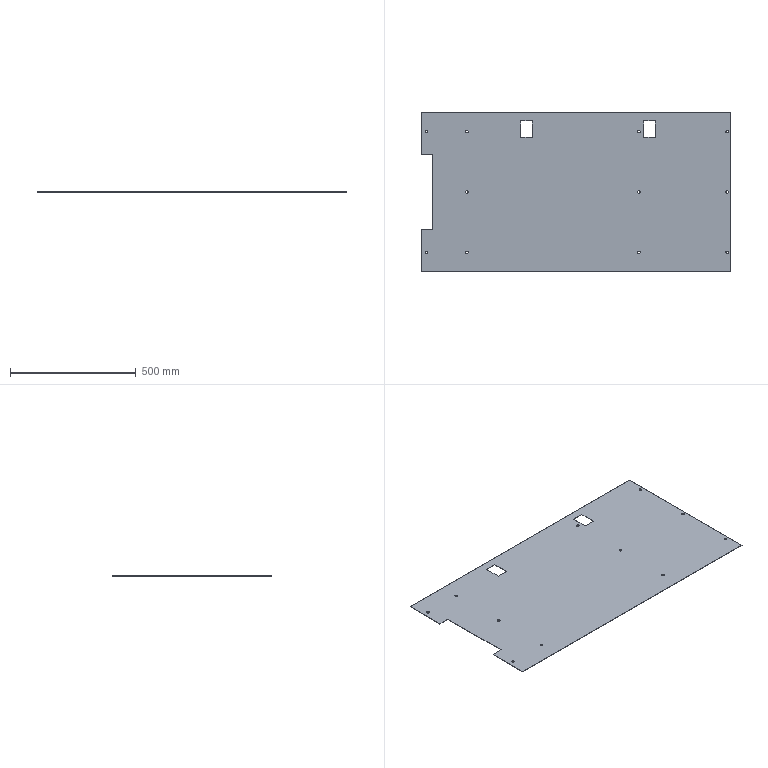Part | STEP file | 1 solid | 40 faces | box 1234 x 636 x 1.5 mm | volume 1146720 mm3 | cylinder 22 | plane 18 | commonest cylinder face diameters 10 x22